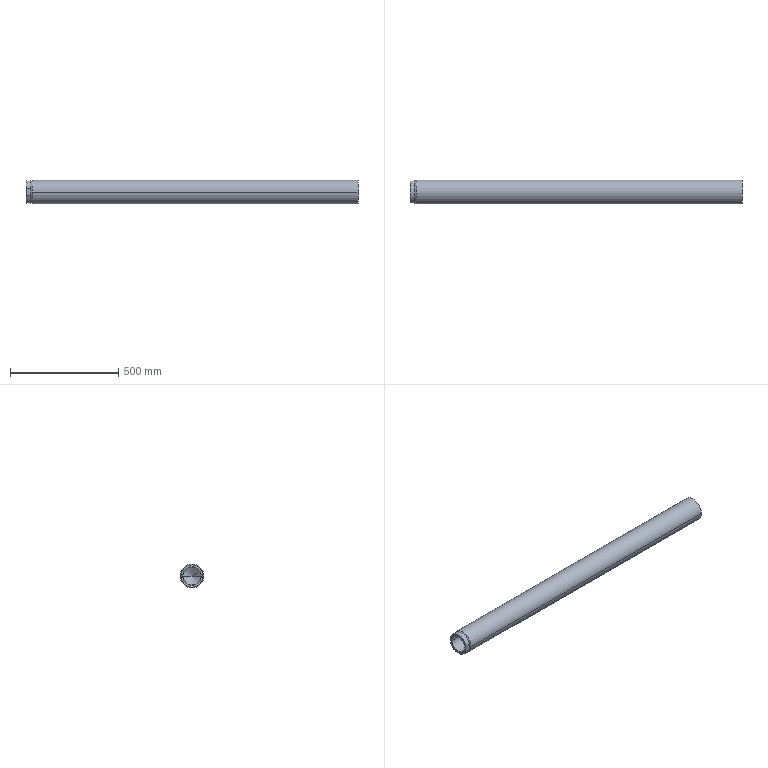Part | SolidWorks | features BaseBody 1 | 1 solid | 25 faces | box 1535 x 110 x 110 mm | volume 13745437 mm3 | cone 10 | cylinder 8 | plane 7 | commonest cylinder face diameters 81.753 x4 104.5 x2 110 x2
STEP:
#1=CARTESIAN_POINT('',(-33.376,40.876,0.));
#2=VERTEX_POINT('',#1);
#3=CARTESIAN_POINT('',(-33.376,-40.876,0.));
#4=VERTEX_POINT('',#3);
#5=CARTESIAN_POINT('',(-33.376,0.,0.));
#6=DIRECTION('',(1.,0.,0.));
#7=DIRECTION('',(0.,1.,0.));
#8=AXIS2_PLACEMENT_3D('',#5,#6,#7);
#9=CIRCLE('',#8,40.876);
#10=EDGE_CURVE('',#2,#4,#9,.T.);
#11=ORIENTED_EDGE('',*,*,#10,.T.);
#12=CARTESIAN_POINT('',(-35.,-42.5,0.));
#13=VERTEX_POINT('',#12);
#14=CARTESIAN_POINT('',(-34.188,-41.688,0.));
#15=DIRECTION('',(-0.7071,-0.7071,0.));
#16=VECTOR('',#15,1000.);
#17=LINE('',#14,#16);
#18=EDGE_CURVE('',#4,#13,#17,.T.);
#19=ORIENTED_EDGE('',*,*,#18,.T.);
#20=CARTESIAN_POINT('',(-35.,42.5,0.));
#21=VERTEX_POINT('',#20);
#22=CARTESIAN_POINT('',(-35.,0.,0.));
#23=DIRECTION('',(1.,0.,0.));
#24=DIRECTION('',(0.,1.,0.));
#25=AXIS2_PLACEMENT_3D('',#22,#23,#24);
#26=CIRCLE('',#25,42.5);
#27=EDGE_CURVE('',#21,#13,#26,.T.);
#28=ORIENTED_EDGE('',*,*,#27,.F.);
#29=CARTESIAN_POINT('',(-34.188,41.688,0.));
#30=DIRECTION('',(-0.7071,0.7071,0.));
#31=VECTOR('',#30,1000.);
#32=LINE('',#29,#31);
#33=EDGE_CURVE('',#2,#21,#32,.T.);
#34=ORIENTED_EDGE('',*,*,#33,.F.);
#35=EDGE_LOOP('',(#11,#19,#28,#34));
#36=FACE_OUTER_BOUND('',#35,.T.);
#37=CARTESIAN_POINT('',(-34.188,0.,0.));
#38=DIRECTION('',(-1.,0.,0.));
#39=DIRECTION('',(0.,1.,0.));
#40=AXIS2_PLACEMENT_3D('',#37,#38,#39);
#41=CONICAL_SURFACE('',#40,41.688,0.7854);
#42=ADVANCED_FACE('',(#36),#41,.F.);
#43=CARTESIAN_POINT('',(70.,40.876,0.));
#44=VERTEX_POINT('',#43);
#45=CARTESIAN_POINT('',(70.,-40.876,0.));
#46=VERTEX_POINT('',#45);
#47=CARTESIAN_POINT('',(70.,0.,0.));
#48=DIRECTION('',(1.,0.,0.));
#49=DIRECTION('',(0.,1.,0.));
#50=AXIS2_PLACEMENT_3D('',#47,#48,#49);
#51=CIRCLE('',#50,40.876);
#52=EDGE_CURVE('',#44,#46,#51,.T.);
#53=ORIENTED_EDGE('',*,*,#52,.T.);
#54=CARTESIAN_POINT('',(18.312,-40.876,0.));
#55=DIRECTION('',(-1.,0.,0.));
#56=VECTOR('',#55,1000.);
#57=LINE('',#54,#56);
#58=EDGE_CURVE('',#46,#4,#57,.T.);
#59=ORIENTED_EDGE('',*,*,#58,.T.);
#60=ORIENTED_EDGE('',*,*,#10,.F.);
#61=CARTESIAN_POINT('',(18.312,40.876,0.));
#62=DIRECTION('',(-1.,0.,0.));
#63=VECTOR('',#62,1000.);
#64=LINE('',#61,#63);
#65=EDGE_CURVE('',#44,#2,#64,.T.);
#66=ORIENTED_EDGE('',*,*,#65,.F.);
#67=EDGE_LOOP('',(#53,#59,#60,#66));
#68=FACE_OUTER_BOUND('',#67,.T.);
#69=CARTESIAN_POINT('',(18.312,0.,0.));
#70=DIRECTION('',(-1.,0.,0.));
#71=DIRECTION('',(0.,1.,0.));
#72=AXIS2_PLACEMENT_3D('',#69,#70,#71);
#73=CYLINDRICAL_SURFACE('',#72,40.876);
#74=ADVANCED_FACE('',(#68),#73,.F.);
#75=CARTESIAN_POINT('',(71.624,40.876,0.));
#76=VERTEX_POINT('',#75);
#77=CARTESIAN_POINT('',(71.624,-40.876,0.));
#78=VERTEX_POINT('',#77);
#79=CARTESIAN_POINT('',(71.624,0.,0.));
#80=DIRECTION('',(1.,0.,0.));
#81=DIRECTION('',(0.,1.,0.));
#82=AXIS2_PLACEMENT_3D('',#79,#80,#81);
#83=CIRCLE('',#82,40.876);
#84=EDGE_CURVE('',#76,#78,#83,.T.);
#85=ORIENTED_EDGE('',*,*,#84,.T.);
#86=CARTESIAN_POINT('',(70.,-42.5,0.));
#87=VERTEX_POINT('',#86);
#88=CARTESIAN_POINT('',(70.812,-41.688,0.));
#89=DIRECTION('',(-0.7071,-0.7071,0.));
#90=VECTOR('',#89,1000.);
#91=LINE('',#88,#90);
#92=EDGE_CURVE('',#78,#87,#91,.T.);
#93=ORIENTED_EDGE('',*,*,#92,.T.);
#94=CARTESIAN_POINT('',(70.,42.5,0.));
#95=VERTEX_POINT('',#94);
#96=CARTESIAN_POINT('',(70.,0.,0.));
#97=DIRECTION('',(1.,0.,0.));
#98=DIRECTION('',(0.,1.,0.));
#99=AXIS2_PLACEMENT_3D('',#96,#97,#98);
#100=CIRCLE('',#99,42.5);
#101=EDGE_CURVE('',#95,#87,#100,.T.);
#102=ORIENTED_EDGE('',*,*,#101,.F.);
#103=CARTESIAN_POINT('',(70.812,41.688,0.));
#104=DIRECTION('',(-0.7071,0.7071,0.));
#105=VECTOR('',#104,1000.);
#106=LINE('',#103,#105);
#107=EDGE_CURVE('',#76,#95,#106,.T.);
#108=ORIENTED_EDGE('',*,*,#107,.F.);
#109=EDGE_LOOP('',(#85,#93,#102,#108));
#110=FACE_OUTER_BOUND('',#109,.T.);
#111=CARTESIAN_POINT('',(70.812,0.,0.));
#112=DIRECTION('',(-1.,0.,0.));
#113=DIRECTION('',(0.,1.,0.));
#114=AXIS2_PLACEMENT_3D('',#111,#112,#113);
#115=CONICAL_SURFACE('',#114,41.688,0.7854);
#116=ADVANCED_FACE('',(#110),#115,.F.);
#117=CARTESIAN_POINT('',(112.5,40.876,0.));
#118=VERTEX_POINT('',#117);
#119=CARTESIAN_POINT('',(112.5,-40.876,0.));
#120=VERTEX_POINT('',#119);
#121=CARTESIAN_POINT('',(112.5,0.,0.));
#122=DIRECTION('',(1.,0.,0.));
#123=DIRECTION('',(0.,1.,0.));
#124=AXIS2_PLACEMENT_3D('',#121,#122,#123);
#125=CIRCLE('',#124,40.876);
#126=EDGE_CURVE('',#118,#120,#125,.T.);
#127=ORIENTED_EDGE('',*,*,#126,.T.);
#128=CARTESIAN_POINT('',(92.062,-40.876,0.));
#129=DIRECTION('',(-1.,0.,0.));
#130=VECTOR('',#129,1000.);
#131=LINE('',#128,#130);
#132=EDGE_CURVE('',#120,#78,#131,.T.);
#133=ORIENTED_EDGE('',*,*,#132,.T.);
#134=ORIENTED_EDGE('',*,*,#84,.F.);
#135=CARTESIAN_POINT('',(92.062,40.876,0.));
#136=DIRECTION('',(-1.,0.,0.));
#137=VECTOR('',#136,1000.);
#138=LINE('',#135,#137);
#139=EDGE_CURVE('',#118,#76,#138,.T.);
#140=ORIENTED_EDGE('',*,*,#139,.F.);
#141=EDGE_LOOP('',(#127,#133,#134,#140));
#142=FACE_OUTER_BOUND('',#141,.T.);
#143=CARTESIAN_POINT('',(92.062,0.,0.));
#144=DIRECTION('',(-1.,0.,0.));
#145=DIRECTION('',(0.,1.,0.));
#146=AXIS2_PLACEMENT_3D('',#143,#144,#145);
#147=CYLINDRICAL_SURFACE('',#146,40.876);
#148=ADVANCED_FACE('',(#142),#147,.F.);
#149=CARTESIAN_POINT('',(136.1,0.,0.));
#150=VERTEX_POINT('',#149);
#151=CARTESIAN_POINT('',(124.3,20.438,0.));
#152=DIRECTION('',(-0.5,0.866,0.));
#153=VECTOR('',#152,1000.);
#154=LINE('',#151,#153);
#155=EDGE_CURVE('',#150,#118,#154,.T.);
#156=ORIENTED_EDGE('',*,*,#155,.F.);
#157=CARTESIAN_POINT('',(124.3,-20.438,0.));
#158=DIRECTION('',(-0.5,-0.866,0.));
#159=VECTOR('',#158,1000.);
#160=LINE('',#157,#159);
#161=EDGE_CURVE('',#150,#120,#160,.T.);
#162=ORIENTED_EDGE('',*,*,#161,.T.);
#163=ORIENTED_EDGE('',*,*,#126,.F.);
#164=EDGE_LOOP('',(#156,#162,#163));
#165=FACE_OUTER_BOUND('',#164,.T.);
#166=CARTESIAN_POINT('',(124.3,0.,0.));
#167=DIRECTION('',(-1.,0.,0.));
#168=DIRECTION('',(0.,1.,0.));
#169=AXIS2_PLACEMENT_3D('',#166,#167,#168);
#170=CONICAL_SURFACE('',#169,20.438,1.047);
#171=ADVANCED_FACE('',(#165),#170,.F.);
#172=CARTESIAN_POINT('',(-6.3,-55.,0.));
#173=VERTEX_POINT('',#172);
#174=CARTESIAN_POINT('',(-6.3,55.,0.));
#175=VERTEX_POINT('',#174);
#176=CARTESIAN_POINT('',(-6.3,0.,0.));
#177=DIRECTION('',(-1.,0.,0.));
#178=DIRECTION('',(0.,1.,0.));
#179=AXIS2_PLACEMENT_3D('',#176,#177,#178);
#180=CIRCLE('',#179,55.);
#181=EDGE_CURVE('',#173,#175,#180,.T.);
#182=ORIENTED_EDGE('',*,*,#181,.F.);
#183=CARTESIAN_POINT('',(1500.,-55.,0.));
#184=VERTEX_POINT('',#183);
#185=CARTESIAN_POINT('',(746.85,-55.,0.));
#186=DIRECTION('',(1.,0.,0.));
#187=VECTOR('',#186,1000.);
#188=LINE('',#185,#187);
#189=EDGE_CURVE('',#173,#184,#188,.T.);
#190=ORIENTED_EDGE('',*,*,#189,.T.);
#191=CARTESIAN_POINT('',(1500.,55.,0.));
#192=VERTEX_POINT('',#191);
#193=CARTESIAN_POINT('',(1500.,0.,0.));
#194=DIRECTION('',(-1.,0.,0.));
#195=DIRECTION('',(0.,1.,0.));
#196=AXIS2_PLACEMENT_3D('',#193,#194,#195);
#197=CIRCLE('',#196,55.);
#198=EDGE_CURVE('',#184,#192,#197,.T.);
#199=ORIENTED_EDGE('',*,*,#198,.T.);
#200=CARTESIAN_POINT('',(746.85,55.,0.));
#201=DIRECTION('',(1.,0.,0.));
#202=VECTOR('',#201,1000.);
#203=LINE('',#200,#202);
#204=EDGE_CURVE('',#175,#192,#203,.T.);
#205=ORIENTED_EDGE('',*,*,#204,.F.);
#206=EDGE_LOOP('',(#182,#190,#199,#205));
#207=FACE_OUTER_BOUND('',#206,.T.);
#208=CARTESIAN_POINT('',(746.85,0.,0.));
#209=DIRECTION('',(1.,0.,0.));
#210=DIRECTION('',(0.,1.,0.));
#211=AXIS2_PLACEMENT_3D('',#208,#209,#210);
#212=CYLINDRICAL_SURFACE('',#211,55.);
#213=ADVANCED_FACE('',(#207),#212,.T.);
#214=CARTESIAN_POINT('',(-12.25,-52.25,0.));
#215=VERTEX_POINT('',#214);
#216=CARTESIAN_POINT('',(-12.25,-50.025,15.085));
#217=VERTEX_POINT('',#216);
#218=CARTESIAN_POINT('',(-12.25,0.,0.));
#219=DIRECTION('',(-1.,0.,0.));
#220=DIRECTION('',(0.,1.,0.));
#221=AXIS2_PLACEMENT_3D('',#218,#219,#220);
#222=CIRCLE('',#221,52.25);
#223=EDGE_CURVE('',#215,#217,#222,.T.);
#224=ORIENTED_EDGE('',*,*,#223,.F.);
#225=CARTESIAN_POINT('',(-9.275,-53.625,0.));
#226=DIRECTION('',(0.9077,-0.4195,0.));
#227=VECTOR('',#226,1000.);
#228=LINE('',#225,#227);
#229=EDGE_CURVE('',#215,#173,#228,.T.);
#230=ORIENTED_EDGE('',*,*,#229,.T.);
#231=ORIENTED_EDGE('',*,*,#181,.T.);
#232=CARTESIAN_POINT('',(-12.25,52.25,0.));
#233=VERTEX_POINT('',#232);
#234=CARTESIAN_POINT('',(-9.275,53.625,0.));
#235=DIRECTION('',(0.9077,0.4195,0.));
#236=VECTOR('',#235,1000.);
#237=LINE('',#234,#236);
#238=EDGE_CURVE('',#233,#175,#237,.T.);
#239=ORIENTED_EDGE('',*,*,#238,.F.);
#240=CARTESIAN_POINT('',(-12.25,50.025,15.085));
#241=VERTEX_POINT('',#240);
#242=CARTESIAN_POINT('',(-12.25,0.,0.));
#243=DIRECTION('',(-1.,0.,0.));
#244=DIRECTION('',(0.,1.,0.));
#245=AXIS2_PLACEMENT_3D('',#242,#243,#244);
#246=CIRCLE('',#245,52.25);
#247=EDGE_CURVE('',#241,#233,#246,.T.);
#248=ORIENTED_EDGE('',*,*,#247,.F.);
#249=CARTESIAN_POINT('',(-12.25,0.,0.));
#250=DIRECTION('',(-1.,0.,0.));
#251=DIRECTION('',(0.,1.,0.));
#252=AXIS2_PLACEMENT_3D('',#249,#250,#251);
#253=CIRCLE('',#252,52.25);
#254=EDGE_CURVE('',#217,#241,#253,.T.);
#255=ORIENTED_EDGE('',*,*,#254,.F.);
#256=EDGE_LOOP('',(#224,#230,#231,#239,#248,#255));
#257=FACE_OUTER_BOUND('',#256,.T.);
#258=CARTESIAN_POINT('',(-9.275,0.,0.));
#259=DIRECTION('',(1.,0.,0.));
#260=DIRECTION('',(0.,1.,0.));
#261=AXIS2_PLACEMENT_3D('',#258,#259,#260);
#262=CONICAL_SURFACE('',#261,53.625,0.4329);
#263=ADVANCED_FACE('',(#257),#262,.T.);
#264=ORIENTED_EDGE('',*,*,#229,.F.);
#265=CARTESIAN_POINT('',(-12.25,-50.025,-15.085));
#266=VERTEX_POINT('',#265);
#267=CARTESIAN_POINT('',(-12.25,0.,0.));
#268=DIRECTION('',(-1.,0.,0.));
#269=DIRECTION('',(0.,1.,0.));
#270=AXIS2_PLACEMENT_3D('',#267,#268,#269);
#271=CIRCLE('',#270,52.25);
#272=EDGE_CURVE('',#266,#215,#271,.T.);
#273=ORIENTED_EDGE('',*,*,#272,.F.);
#274=CARTESIAN_POINT('',(-12.25,50.025,-15.085));
#275=VERTEX_POINT('',#274);
#276=CARTESIAN_POINT('',(-12.25,0.,0.));
#277=DIRECTION('',(-1.,0.,0.));
#278=DIRECTION('',(0.,1.,0.));
#279=AXIS2_PLACEMENT_3D('',#276,#277,#278);
#280=CIRCLE('',#279,52.25);
#281=EDGE_CURVE('',#275,#266,#280,.T.);
#282=ORIENTED_EDGE('',*,*,#281,.F.);
#283=CARTESIAN_POINT('',(-12.25,0.,0.));
#284=DIRECTION('',(-1.,0.,0.));
#285=DIRECTION('',(0.,1.,0.));
#286=AXIS2_PLACEMENT_3D('',#283,#284,#285);
#287=CIRCLE('',#286,52.25);
#288=EDGE_CURVE('',#233,#275,#287,.T.);
#289=ORIENTED_EDGE('',*,*,#288,.F.);
#290=ORIENTED_EDGE('',*,*,#238,.T.);
#291=CARTESIAN_POINT('',(-6.3,0.,0.));
#292=DIRECTION('',(-1.,0.,0.));
#293=DIRECTION('',(0.,1.,0.));
#294=AXIS2_PLACEMENT_3D('',#291,#292,#293);
#295=CIRCLE('',#294,55.);
#296=EDGE_CURVE('',#175,#173,#295,.T.);
#297=ORIENTED_EDGE('',*,*,#296,.T.);
#298=EDGE_LOOP('',(#264,#273,#282,#289,#290,#297));
#299=FACE_OUTER_BOUND('',#298,.T.);
#300=CARTESIAN_POINT('',(-9.275,0.,0.));
#301=DIRECTION('',(1.,0.,0.));
#302=DIRECTION('',(0.,1.,0.));
#303=AXIS2_PLACEMENT_3D('',#300,#301,#302);
#304=CONICAL_SURFACE('',#303,53.625,0.4329);
#305=ADVANCED_FACE('',(#299),#304,.T.);
#306=ORIENTED_EDGE('',*,*,#189,.F.);
#307=ORIENTED_EDGE('',*,*,#296,.F.);
#308=ORIENTED_EDGE('',*,*,#204,.T.);
#309=CARTESIAN_POINT('',(1500.,0.,0.));
#310=DIRECTION('',(-1.,0.,0.));
#311=DIRECTION('',(0.,1.,0.));
#312=AXIS2_PLACEMENT_3D('',#309,#310,#311);
#313=CIRCLE('',#312,55.);
#314=EDGE_CURVE('',#192,#184,#313,.T.);
#315=ORIENTED_EDGE('',*,*,#314,.T.);
#316=EDGE_LOOP('',(#306,#307,#308,#315));
#317=FACE_OUTER_BOUND('',#316,.T.);
#318=CARTESIAN_POINT('',(746.85,0.,0.));
#319=DIRECTION('',(1.,0.,0.));
#320=DIRECTION('',(0.,1.,0.));
#321=AXIS2_PLACEMENT_3D('',#318,#319,#320);
#322=CYLINDRICAL_SURFACE('',#321,55.);
#323=ADVANCED_FACE('',(#317),#322,.T.);
#324=ORIENTED_EDGE('',*,*,#314,.F.);
#325=ORIENTED_EDGE('',*,*,#198,.F.);
#326=EDGE_LOOP('',(#324,#325));
#327=FACE_OUTER_BOUND('',#326,.T.);
#328=CARTESIAN_POINT('',(1500.,27.5,0.));
#329=DIRECTION('',(1.,0.,0.));
#330=DIRECTION('',(0.,-1.,0.));
#331=AXIS2_PLACEMENT_3D('',#328,#329,#330);
#332=PLANE('',#331);
#333=ADVANCED_FACE('',(#327),#332,.T.);
#334=ORIENTED_EDGE('',*,*,#161,.F.);
#335=ORIENTED_EDGE('',*,*,#155,.T.);
#336=CARTESIAN_POINT('',(112.5,0.,0.));
#337=DIRECTION('',(1.,0.,0.));
#338=DIRECTION('',(0.,1.,0.));
#339=AXIS2_PLACEMENT_3D('',#336,#337,#338);
#340=CIRCLE('',#339,40.876);
#341=EDGE_CURVE('',#120,#118,#340,.T.);
#342=ORIENTED_EDGE('',*,*,#341,.F.);
#343=EDGE_LOOP('',(#334,#335,#342));
#344=FACE_OUTER_BOUND('',#343,.T.);
#345=CARTESIAN_POINT('',(124.3,0.,0.));
#346=DIRECTION('',(-1.,0.,0.));
#347=DIRECTION('',(0.,1.,0.));
#348=AXIS2_PLACEMENT_3D('',#345,#346,#347);
#349=CONICAL_SURFACE('',#348,20.438,1.047);
#350=ADVANCED_FACE('',(#344),#349,.F.);
#351=ORIENTED_EDGE('',*,*,#132,.F.);
#352=ORIENTED_EDGE('',*,*,#341,.T.);
#353=ORIENTED_EDGE('',*,*,#139,.T.);
#354=CARTESIAN_POINT('',(71.624,0.,0.));
#355=DIRECTION('',(1.,0.,0.));
#356=DIRECTION('',(0.,1.,0.));
#357=AXIS2_PLACEMENT_3D('',#354,#355,#356);
#358=CIRCLE('',#357,40.876);
#359=EDGE_CURVE('',#78,#76,#358,.T.);
#360=ORIENTED_EDGE('',*,*,#359,.F.);
#361=EDGE_LOOP('',(#351,#352,#353,#360));
#362=FACE_OUTER_BOUND('',#361,.T.);
#363=CARTESIAN_POINT('',(92.062,0.,0.));
#364=DIRECTION('',(-1.,0.,0.));
#365=DIRECTION('',(0.,1.,0.));
#366=AXIS2_PLACEMENT_3D('',#363,#364,#365);
#367=CYLINDRICAL_SURFACE('',#366,40.876);
#368=ADVANCED_FACE('',(#362),#367,.F.);
#369=ORIENTED_EDGE('',*,*,#92,.F.);
#370=ORIENTED_EDGE('',*,*,#359,.T.);
#371=ORIENTED_EDGE('',*,*,#107,.T.);
#372=CARTESIAN_POINT('',(70.,0.,0.));
#373=DIRECTION('',(1.,0.,0.));
#374=DIRECTION('',(0.,1.,0.));
#375=AXIS2_PLACEMENT_3D('',#372,#373,#374);
#376=CIRCLE('',#375,42.5);
#377=EDGE_CURVE('',#87,#95,#376,.T.);
#378=ORIENTED_EDGE('',*,*,#377,.F.);
#379=EDGE_LOOP('',(#369,#370,#371,#378));
#380=FACE_OUTER_BOUND('',#379,.T.);
#381=CARTESIAN_POINT('',(70.812,0.,0.));
#382=DIRECTION('',(-1.,0.,0.));
#383=DIRECTION('',(0.,1.,0.));
#384=AXIS2_PLACEMENT_3D('',#381,#382,#383);
#385=CONICAL_SURFACE('',#384,41.688,0.7854);
#386=ADVANCED_FACE('',(#380),#385,.F.);
#387=ORIENTED_EDGE('',*,*,#52,.F.);
#388=CARTESIAN_POINT('',(70.,0.,0.));
#389=DIRECTION('',(1.,0.,0.));
#390=DIRECTION('',(0.,1.,0.));
#391=AXIS2_PLACEMENT_3D('',#388,#389,#390);
#392=CIRCLE('',#391,40.876);
#393=EDGE_CURVE('',#46,#44,#392,.T.);
#394=ORIENTED_EDGE('',*,*,#393,.F.);
#395=EDGE_LOOP('',(#387,#394));
#396=FACE_BOUND('',#395,.T.);
#397=ORIENTED_EDGE('',*,*,#101,.T.);
#398=ORIENTED_EDGE('',*,*,#377,.T.);
#399=EDGE_LOOP('',(#397,#398));
#400=FACE_OUTER_BOUND('',#399,.T.);
#401=CARTESIAN_POINT('',(70.,41.688,0.));
#402=DIRECTION('',(-1.,0.,0.));
#403=DIRECTION('',(0.,-1.,0.));
#404=AXIS2_PLACEMENT_3D('',#401,#402,#403);
#405=PLANE('',#404);
#406=ADVANCED_FACE('',(#396,#400),#405,.F.);
#407=ORIENTED_EDGE('',*,*,#58,.F.);
#408=ORIENTED_EDGE('',*,*,#393,.T.);
#409=ORIENTED_EDGE('',*,*,#65,.T.);
#410=CARTESIAN_POINT('',(-33.376,0.,0.));
#411=DIRECTION('',(1.,0.,0.));
#412=DIRECTION('',(0.,1.,0.));
#413=AXIS2_PLACEMENT_3D('',#410,#411,#412);
#414=CIRCLE('',#413,40.876);
#415=EDGE_CURVE('',#4,#2,#414,.T.);
#416=ORIENTED_EDGE('',*,*,#415,.F.);
#417=EDGE_LOOP('',(#407,#408,#409,#416));
#418=FACE_OUTER_BOUND('',#417,.T.);
#419=CARTESIAN_POINT('',(18.312,0.,0.));
#420=DIRECTION('',(-1.,0.,0.));
#421=DIRECTION('',(0.,1.,0.));
#422=AXIS2_PLACEMENT_3D('',#419,#420,#421);
#423=CYLINDRICAL_SURFACE('',#422,40.876);
#424=ADVANCED_FACE('',(#418),#423,.F.);
#425=ORIENTED_EDGE('',*,*,#18,.F.);
#426=ORIENTED_EDGE('',*,*,#415,.T.);
#427=ORIENTED_EDGE('',*,*,#33,.T.);
#428=CARTESIAN_POINT('',(-35.,0.,0.));
#429=DIRECTION('',(1.,0.,0.));
#430=DIRECTION('',(0.,1.,0.));
#431=AXIS2_PLACEMENT_3D('',#428,#429,#430);
#432=CIRCLE('',#431,42.5);
#433=EDGE_CURVE('',#13,#21,#432,.T.);
#434=ORIENTED_EDGE('',*,*,#433,.F.);
#435=EDGE_LOOP('',(#425,#426,#427,#434));
#436=FACE_OUTER_BOUND('',#435,.T.);
#437=CARTESIAN_POINT('',(-34.188,0.,0.));
#438=DIRECTION('',(-1.,0.,0.));
#439=DIRECTION('',(0.,1.,0.));
#440=AXIS2_PLACEMENT_3D('',#437,#438,#439);
#441=CONICAL_SURFACE('',#440,41.688,0.7854);
#442=ADVANCED_FACE('',(#436),#441,.F.);
#443=CARTESIAN_POINT('',(-34.65,-50.025,-15.085));
#444=VERTEX_POINT('',#443);
#445=CARTESIAN_POINT('',(-23.45,-50.025,-15.085));
#446=DIRECTION('',(-1.,0.,0.));
#447=VECTOR('',#446,1000.);
#448=LINE('',#445,#447);
#449=EDGE_CURVE('',#266,#444,#448,.T.);
#450=ORIENTED_EDGE('',*,*,#449,.T.);
#451=CARTESIAN_POINT('',(-34.65,50.025,-15.085));
#452=VERTEX_POINT('',#451);
#453=CARTESIAN_POINT('',(-34.65,0.,0.));
#454=DIRECTION('',(-1.,0.,0.));
#455=DIRECTION('',(0.,1.,0.));
#456=AXIS2_PLACEMENT_3D('',#453,#454,#455);
#457=CIRCLE('',#456,52.25);
#458=EDGE_CURVE('',#452,#444,#457,.T.);
#459=ORIENTED_EDGE('',*,*,#458,.F.);
#460=CARTESIAN_POINT('',(-23.45,50.025,-15.085));
#461=DIRECTION('',(1.,0.,0.));
#462=VECTOR('',#461,1000.);
#463=LINE('',#460,#462);
#464=EDGE_CURVE('',#452,#275,#463,.T.);
#465=ORIENTED_EDGE('',*,*,#464,.T.);
#466=ORIENTED_EDGE('',*,*,#281,.T.);
#467=EDGE_LOOP('',(#450,#459,#465,#466));
#468=FACE_OUTER_BOUND('',#467,.T.);
#469=CARTESIAN_POINT('',(-23.45,0.,0.));
#470=DIRECTION('',(1.,0.,0.));
#471=DIRECTION('',(0.,1.,0.));
#472=AXIS2_PLACEMENT_3D('',#469,#470,#471);
#473=CYLINDRICAL_SURFACE('',#472,52.25);
#474=ADVANCED_FACE('',(#468),#473,.T.);
#475=CARTESIAN_POINT('',(-35.,50.025,-13.824));
#476=VERTEX_POINT('',#475);
#477=CARTESIAN_POINT('',(-35.,50.025,-13.824));
#478=CARTESIAN_POINT('',(-34.833,50.025,-14.453));
#479=CARTESIAN_POINT('',(-34.65,50.025,-15.085));
#480=(BOUNDED_CURVE()B_SPLINE_CURVE(2,(#477,#478,#479),.UNSPECIFIED.,.F.,.F.)B_SPLINE_CURVE_WITH_KNOTS((3,3),(0.,1.309),.UNSPECIFIED.)CURVE()GEOMETRIC_REPRESENTATION_ITEM()RATIONAL_B_SPLINE_CURVE((1.,1.,1.))REPRESENTATION_ITEM(''));
#481=EDGE_CURVE('',#476,#452,#480,.T.);
#482=ORIENTED_EDGE('',*,*,#481,.F.);
#483=CARTESIAN_POINT('',(-35.,50.025,13.824));
#484=VERTEX_POINT('',#483);
#485=CARTESIAN_POINT('',(-35.,50.025,0.));
#486=DIRECTION('',(0.,0.,-1.));
#487=VECTOR('',#486,1000.);
#488=LINE('',#485,#487);
#489=EDGE_CURVE('',#484,#476,#488,.T.);
#490=ORIENTED_EDGE('',*,*,#489,.F.);
#491=CARTESIAN_POINT('',(-34.65,50.025,15.085));
#492=VERTEX_POINT('',#491);
#493=CARTESIAN_POINT('',(-34.65,50.025,15.085));
#494=CARTESIAN_POINT('',(-34.833,50.025,14.453));
#495=CARTESIAN_POINT('',(-35.,50.025,13.824));
#496=(BOUNDED_CURVE()B_SPLINE_CURVE(2,(#493,#494,#495),.UNSPECIFIED.,.F.,.F.)B_SPLINE_CURVE_WITH_KNOTS((3,3),(0.,1.309),.UNSPECIFIED.)CURVE()GEOMETRIC_REPRESENTATION_ITEM()RATIONAL_B_SPLINE_CURVE((1.,1.,1.))REPRESENTATION_ITEM(''));
#497=EDGE_CURVE('',#492,#484,#496,.T.);
#498=ORIENTED_EDGE('',*,*,#497,.F.);
#499=CARTESIAN_POINT('',(-23.45,50.025,15.085));
#500=DIRECTION('',(-1.,0.,0.));
#501=VECTOR('',#500,1000.);
#502=LINE('',#499,#501);
#503=EDGE_CURVE('',#241,#492,#502,.T.);
#504=ORIENTED_EDGE('',*,*,#503,.F.);
#505=CARTESIAN_POINT('',(-12.25,50.025,0.));
#506=DIRECTION('',(0.,0.,1.));
#507=VECTOR('',#506,1000.);
#508=LINE('',#505,#507);
#509=EDGE_CURVE('',#275,#241,#508,.T.);
#510=ORIENTED_EDGE('',*,*,#509,.F.);
#511=ORIENTED_EDGE('',*,*,#464,.F.);
#512=EDGE_LOOP('',(#482,#490,#498,#504,#510,#511));
#513=FACE_OUTER_BOUND('',#512,.T.);
#514=CARTESIAN_POINT('',(-23.625,50.025,0.));
#515=DIRECTION('',(0.,1.,0.));
#516=DIRECTION('',(0.,0.,-1.));
#517=AXIS2_PLACEMENT_3D('',#514,#515,#516);
#518=PLANE('',#517);
#519=ADVANCED_FACE('',(#513),#518,.T.);
#520=ORIENTED_EDGE('',*,*,#247,.T.);
#521=ORIENTED_EDGE('',*,*,#288,.T.);
#522=ORIENTED_EDGE('',*,*,#509,.T.);
#523=EDGE_LOOP('',(#520,#521,#522));
#524=FACE_OUTER_BOUND('',#523,.T.);
#525=CARTESIAN_POINT('',(-12.25,105.025,0.));
#526=DIRECTION('',(-1.,0.,0.));
#527=DIRECTION('',(0.,0.,1.));
#528=AXIS2_PLACEMENT_3D('',#525,#526,#527);
#529=PLANE('',#528);
#530=ADVANCED_FACE('',(#524),#529,.T.);
#531=CARTESIAN_POINT('',(-34.65,-50.025,15.085));
#532=VERTEX_POINT('',#531);
#533=CARTESIAN_POINT('',(-23.45,-50.025,15.085));
#534=DIRECTION('',(1.,0.,0.));
#535=VECTOR('',#534,1000.);
#536=LINE('',#533,#535);
#537=EDGE_CURVE('',#532,#217,#536,.T.);
#538=ORIENTED_EDGE('',*,*,#537,.T.);
#539=ORIENTED_EDGE('',*,*,#254,.T.);
#540=ORIENTED_EDGE('',*,*,#503,.T.);
#541=CARTESIAN_POINT('',(-34.65,0.,0.));
#542=DIRECTION('',(-1.,0.,0.));
#543=DIRECTION('',(0.,1.,0.));
#544=AXIS2_PLACEMENT_3D('',#541,#542,#543);
#545=CIRCLE('',#544,52.25);
#546=EDGE_CURVE('',#532,#492,#545,.T.);
#547=ORIENTED_EDGE('',*,*,#546,.F.);
#548=EDGE_LOOP('',(#538,#539,#540,#547));
#549=FACE_OUTER_BOUND('',#548,.T.);
#550=CARTESIAN_POINT('',(-23.45,0.,0.));
#551=DIRECTION('',(1.,0.,0.));
#552=DIRECTION('',(0.,1.,0.));
#553=AXIS2_PLACEMENT_3D('',#550,#551,#552);
#554=CYLINDRICAL_SURFACE('',#553,52.25);
#555=ADVANCED_FACE('',(#549),#554,.T.);
#556=CARTESIAN_POINT('',(-35.,-50.025,-13.824));
#557=VERTEX_POINT('',#556);
#558=CARTESIAN_POINT('',(-34.65,-50.025,-15.085));
#559=CARTESIAN_POINT('',(-34.833,-50.025,-14.453));
#560=CARTESIAN_POINT('',(-35.,-50.025,-13.824));
#561=(BOUNDED_CURVE()B_SPLINE_CURVE(2,(#558,#559,#560),.UNSPECIFIED.,.F.,.F.)B_SPLINE_CURVE_WITH_KNOTS((3,3),(0.,1.309),.UNSPECIFIED.)CURVE()GEOMETRIC_REPRESENTATION_ITEM()RATIONAL_B_SPLINE_CURVE((1.,1.,1.))REPRESENTATION_ITEM(''));
#562=EDGE_CURVE('',#444,#557,#561,.T.);
#563=ORIENTED_EDGE('',*,*,#562,.T.);
#564=CARTESIAN_POINT('',(-35.,0.,0.));
#565=DIRECTION('',(-1.,0.,0.));
#566=DIRECTION('',(0.,1.,0.));
#567=AXIS2_PLACEMENT_3D('',#564,#565,#566);
#568=CIRCLE('',#567,51.9);
#569=EDGE_CURVE('',#476,#557,#568,.T.);
#570=ORIENTED_EDGE('',*,*,#569,.F.);
#571=ORIENTED_EDGE('',*,*,#481,.T.);
#572=ORIENTED_EDGE('',*,*,#458,.T.);
#573=EDGE_LOOP('',(#563,#570,#571,#572));
#574=FACE_OUTER_BOUND('',#573,.T.);
#575=CARTESIAN_POINT('',(-34.825,0.,0.));
#576=DIRECTION('',(1.,0.,0.));
#577=DIRECTION('',(0.,1.,0.));
#578=AXIS2_PLACEMENT_3D('',#575,#576,#577);
#579=CONICAL_SURFACE('',#578,52.075,0.7854);
#580=ADVANCED_FACE('',(#574),#579,.T.);
#581=CARTESIAN_POINT('',(-35.,-50.025,13.824));
#582=VERTEX_POINT('',#581);
#583=CARTESIAN_POINT('',(-35.,-50.025,13.824));
#584=CARTESIAN_POINT('',(-34.833,-50.025,14.453));
#585=CARTESIAN_POINT('',(-34.65,-50.025,15.085));
#586=(BOUNDED_CURVE()B_SPLINE_CURVE(2,(#583,#584,#585),.UNSPECIFIED.,.F.,.F.)B_SPLINE_CURVE_WITH_KNOTS((3,3),(0.,1.309),.UNSPECIFIED.)CURVE()GEOMETRIC_REPRESENTATION_ITEM()RATIONAL_B_SPLINE_CURVE((1.,1.,1.))REPRESENTATION_ITEM(''));
#587=EDGE_CURVE('',#582,#532,#586,.T.);
#588=ORIENTED_EDGE('',*,*,#587,.T.);
#589=ORIENTED_EDGE('',*,*,#546,.T.);
#590=ORIENTED_EDGE('',*,*,#497,.T.);
#591=CARTESIAN_POINT('',(-35.,0.,0.));
#592=DIRECTION('',(-1.,0.,0.));
#593=DIRECTION('',(0.,1.,0.));
#594=AXIS2_PLACEMENT_3D('',#591,#592,#593);
#595=CIRCLE('',#594,51.9);
#596=EDGE_CURVE('',#582,#484,#595,.T.);
#597=ORIENTED_EDGE('',*,*,#596,.F.);
#598=EDGE_LOOP('',(#588,#589,#590,#597));
#599=FACE_OUTER_BOUND('',#598,.T.);
#600=CARTESIAN_POINT('',(-34.825,0.,0.));
#601=DIRECTION('',(1.,0.,0.));
#602=DIRECTION('',(0.,1.,0.));
#603=AXIS2_PLACEMENT_3D('',#600,#601,#602);
#604=CONICAL_SURFACE('',#603,52.075,0.7854);
#605=ADVANCED_FACE('',(#599),#604,.T.);
#606=CARTESIAN_POINT('',(-35.,-50.025,0.));
#607=DIRECTION('',(0.,0.,1.));
#608=VECTOR('',#607,1000.);
#609=LINE('',#606,#608);
#610=EDGE_CURVE('',#557,#582,#609,.T.);
#611=ORIENTED_EDGE('',*,*,#610,.T.);
#612=ORIENTED_EDGE('',*,*,#596,.T.);
#613=ORIENTED_EDGE('',*,*,#489,.T.);
#614=ORIENTED_EDGE('',*,*,#569,.T.);
#615=EDGE_LOOP('',(#611,#612,#613,#614));
#616=FACE_OUTER_BOUND('',#615,.T.);
#617=ORIENTED_EDGE('',*,*,#27,.T.);
#618=ORIENTED_EDGE('',*,*,#433,.T.);
#619=EDGE_LOOP('',(#617,#618));
#620=FACE_BOUND('',#619,.T.);
#621=CARTESIAN_POINT('',(-35.,25.95,0.));
#622=DIRECTION('',(-1.,0.,0.));
#623=DIRECTION('',(0.,1.,0.));
#624=AXIS2_PLACEMENT_3D('',#621,#622,#623);
#625=PLANE('',#624);
#626=ADVANCED_FACE('',(#616,#620),#625,.T.);
#627=ORIENTED_EDGE('',*,*,#272,.T.);
#628=ORIENTED_EDGE('',*,*,#223,.T.);
#629=CARTESIAN_POINT('',(-12.25,-50.025,0.));
#630=DIRECTION('',(0.,0.,-1.));
#631=VECTOR('',#630,1000.);
#632=LINE('',#629,#631);
#633=EDGE_CURVE('',#217,#266,#632,.T.);
#634=ORIENTED_EDGE('',*,*,#633,.T.);
#635=EDGE_LOOP('',(#627,#628,#634));
#636=FACE_OUTER_BOUND('',#635,.T.);
#637=CARTESIAN_POINT('',(-12.25,-105.025,0.));
#638=DIRECTION('',(-1.,0.,0.));
#639=DIRECTION('',(0.,0.,-1.));
#640=AXIS2_PLACEMENT_3D('',#637,#638,#639);
#641=PLANE('',#640);
#642=ADVANCED_FACE('',(#636),#641,.T.);
#643=ORIENTED_EDGE('',*,*,#562,.F.);
#644=ORIENTED_EDGE('',*,*,#449,.F.);
#645=ORIENTED_EDGE('',*,*,#633,.F.);
#646=ORIENTED_EDGE('',*,*,#537,.F.);
#647=ORIENTED_EDGE('',*,*,#587,.F.);
#648=ORIENTED_EDGE('',*,*,#610,.F.);
#649=EDGE_LOOP('',(#643,#644,#645,#646,#647,#648));
#650=FACE_OUTER_BOUND('',#649,.T.);
#651=CARTESIAN_POINT('',(-23.625,-50.025,0.));
#652=DIRECTION('',(0.,-1.,0.));
#653=DIRECTION('',(0.,0.,1.));
#654=AXIS2_PLACEMENT_3D('',#651,#652,#653);
#655=PLANE('',#654);
#656=ADVANCED_FACE('',(#650),#655,.T.);
#657=CLOSED_SHELL('',(#42,#74,#116,#148,#171,#213,#263,#305,#323,#333,#350,#368,#386,#406,#424,#442,#474,#519,#530,#555,#580,#605,#626,#642,#656));
#658=MANIFOLD_SOLID_BREP('',#657);
#659=CARTESIAN_POINT('',(0.,0.,0.));
#660=DIRECTION('',(0.,0.,1.));
#661=DIRECTION('',(1.,0.,0.));
#662=AXIS2_PLACEMENT_3D('',#659,#660,#661);
#663=(LENGTH_UNIT()NAMED_UNIT(*)SI_UNIT(.MILLI.,.METRE.));
#664=UNCERTAINTY_MEASURE_WITH_UNIT(LENGTH_MEASURE(0.00001),#663,'','');
#665=(NAMED_UNIT(*)PLANE_ANGLE_UNIT()SI_UNIT($,.RADIAN.));
#666=(NAMED_UNIT(*)SI_UNIT($,.STERADIAN.)SOLID_ANGLE_UNIT());
#667=(GEOMETRIC_REPRESENTATION_CONTEXT(3)GLOBAL_UNCERTAINTY_ASSIGNED_CONTEXT((#664))GLOBAL_UNIT_ASSIGNED_CONTEXT((#663,#665,#666))REPRESENTATION_CONTEXT('',''));
#668=ADVANCED_BREP_SHAPE_REPRESENTATION('',(#658,#662),#667);